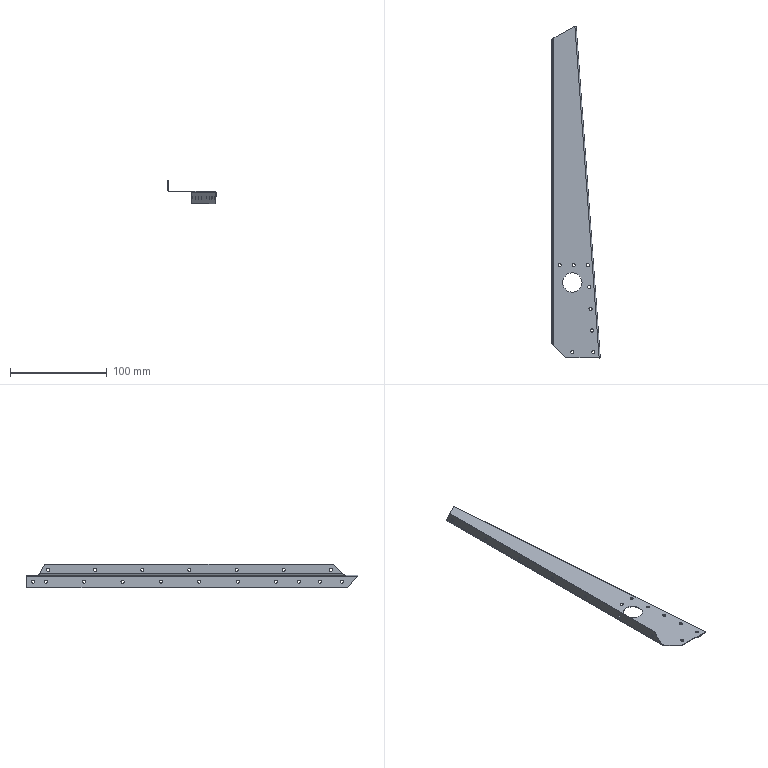Part | SolidWorks | features BaseBody 1 | 1 solid | 79 faces | box 50.137 x 342.625 x 24.641 mm | volume 9738 mm3 | cylinder 58 | plane 15 | spline 6 | commonest cylinder face diameters 3.2 x52 20 x2 1.6 x1 2.6 x1 3.6 x1 4.6 x1